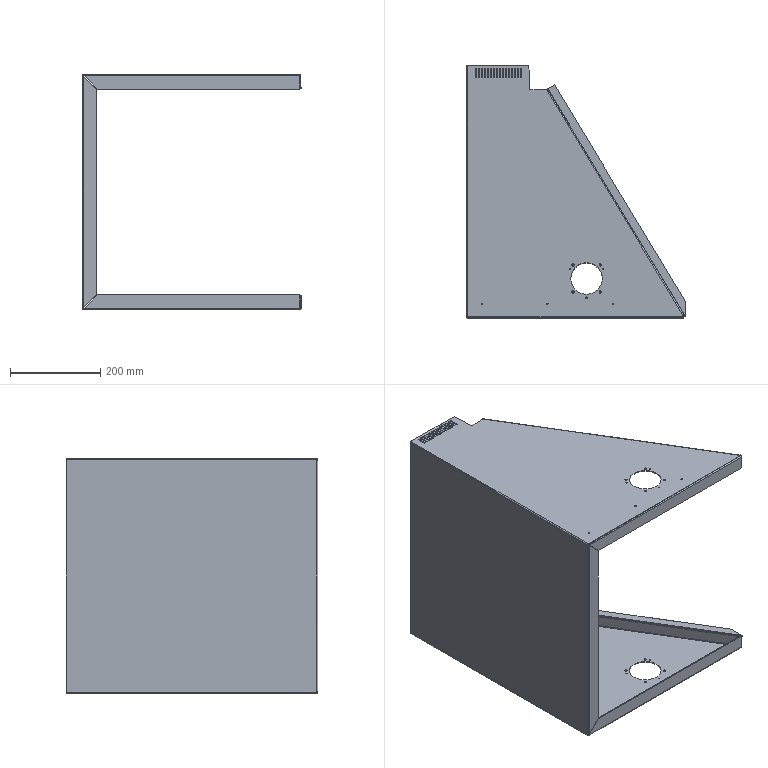Part | SolidWorks | features EdgeFlange 6, ICE 6, FlatPattern 1, SMBaseFlange 1, SMMiteredFlange 1, SheetMetal 1 | 1 solid | 273 faces | box 485.154 x 558 x 520 mm | volume 1443065 mm3 | plane 139 | cylinder 130 | spline 4 | commonest cylinder face diameters 3 x68 3.3 x22 5 x14 1.473 x9 5.473 x9 3.2 x2